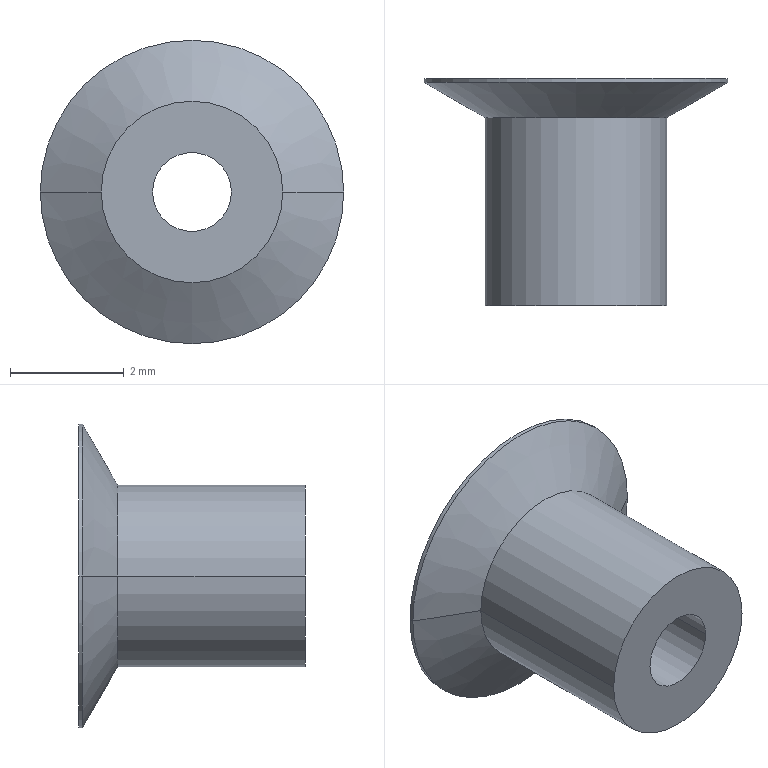Part | NX | features solid 2 | 1 solid | 12 faces | box 5.348 x 4 x 5.348 mm | volume 31.105 mm3 | cylinder 6 | torus 2 | plane 2 | cone 2 | commonest cylinder face diameters 1.39 x2 3.2 x2 5.348 x2
STEP:
#1=CARTESIAN_POINT('',(-257.575,146.75,-216.46));
#2=VERTEX_POINT('',#1);
#3=CARTESIAN_POINT('',(-258.965,146.75,-216.46));
#4=VERTEX_POINT('',#3);
#5=CARTESIAN_POINT('',(-258.27,146.75,-216.46));
#6=DIRECTION('',(0.,1.,0.));
#7=DIRECTION('',(1.,0.,0.));
#8=AXIS2_PLACEMENT_3D('',#5,#6,#7);
#9=CIRCLE('',#8,0.695);
#10=EDGE_CURVE('',#2,#4,#9,.T.);
#11=ORIENTED_EDGE('',*,*,#10,.T.);
#12=CARTESIAN_POINT('',(-258.965,143.06,-216.46));
#13=VERTEX_POINT('',#12);
#14=CARTESIAN_POINT('',(-258.965,146.75,-216.46));
#15=DIRECTION('',(0.,-1.,0.));
#16=VECTOR('',#15,1000.);
#17=LINE('',#14,#16);
#18=EDGE_CURVE('',#4,#13,#17,.T.);
#19=ORIENTED_EDGE('',*,*,#18,.T.);
#20=CARTESIAN_POINT('',(-257.575,143.06,-216.46));
#21=VERTEX_POINT('',#20);
#22=CARTESIAN_POINT('',(-258.27,143.06,-216.46));
#23=DIRECTION('',(0.,-1.,0.));
#24=DIRECTION('',(-1.,0.,0.));
#25=AXIS2_PLACEMENT_3D('',#22,#23,#24);
#26=CIRCLE('',#25,0.695);
#27=EDGE_CURVE('',#13,#21,#26,.T.);
#28=ORIENTED_EDGE('',*,*,#27,.T.);
#29=CARTESIAN_POINT('',(-257.575,146.75,-216.46));
#30=DIRECTION('',(0.,-1.,0.));
#31=VECTOR('',#30,1000.);
#32=LINE('',#29,#31);
#33=EDGE_CURVE('',#21,#2,#32,.F.);
#34=ORIENTED_EDGE('',*,*,#33,.T.);
#35=EDGE_LOOP('',(#11,#19,#28,#34));
#36=FACE_BOUND('',#35,.T.);
#37=CARTESIAN_POINT('',(-258.27,141.06,-216.46));
#38=DIRECTION('',(0.,-1.,0.));
#39=DIRECTION('',(1.,0.,0.));
#40=AXIS2_PLACEMENT_3D('',#37,#38,#39);
#41=CYLINDRICAL_SURFACE('',#40,0.695);
#42=ADVANCED_FACE('',(#36),#41,.F.);
#43=ORIENTED_EDGE('',*,*,#33,.F.);
#44=CARTESIAN_POINT('',(-258.27,143.06,-216.46));
#45=DIRECTION('',(0.,-1.,0.));
#46=DIRECTION('',(1.,0.,0.));
#47=AXIS2_PLACEMENT_3D('',#44,#45,#46);
#48=CIRCLE('',#47,0.695);
#49=EDGE_CURVE('',#21,#13,#48,.T.);
#50=ORIENTED_EDGE('',*,*,#49,.T.);
#51=ORIENTED_EDGE('',*,*,#18,.F.);
#52=CARTESIAN_POINT('',(-258.27,146.75,-216.46));
#53=DIRECTION('',(0.,1.,0.));
#54=DIRECTION('',(-1.,0.,0.));
#55=AXIS2_PLACEMENT_3D('',#52,#53,#54);
#56=CIRCLE('',#55,0.695);
#57=EDGE_CURVE('',#4,#2,#56,.T.);
#58=ORIENTED_EDGE('',*,*,#57,.T.);
#59=EDGE_LOOP('',(#43,#50,#51,#58));
#60=FACE_BOUND('',#59,.T.);
#61=CARTESIAN_POINT('',(-258.27,141.06,-216.46));
#62=DIRECTION('',(0.,-1.,0.));
#63=DIRECTION('',(1.,0.,0.));
#64=AXIS2_PLACEMENT_3D('',#61,#62,#63);
#65=CYLINDRICAL_SURFACE('',#64,0.695);
#66=ADVANCED_FACE('',(#60),#65,.F.);
#67=ORIENTED_EDGE('',*,*,#57,.F.);
#68=CARTESIAN_POINT('',(-259.275,147.06,-216.46));
#69=VERTEX_POINT('',#68);
#70=CARTESIAN_POINT('',(-259.275,146.75,-216.46));
#71=DIRECTION('',(0.,0.,1.));
#72=DIRECTION('',(1.,0.,0.));
#73=AXIS2_PLACEMENT_3D('',#70,#71,#72);
#74=CIRCLE('',#73,0.31);
#75=EDGE_CURVE('',#4,#69,#74,.T.);
#76=ORIENTED_EDGE('',*,*,#75,.T.);
#77=CARTESIAN_POINT('',(-257.265,147.06,-216.46));
#78=VERTEX_POINT('',#77);
#79=CARTESIAN_POINT('',(-258.27,147.06,-216.46));
#80=DIRECTION('',(0.,1.,0.));
#81=DIRECTION('',(-1.,0.,0.));
#82=AXIS2_PLACEMENT_3D('',#79,#80,#81);
#83=CIRCLE('',#82,1.005);
#84=EDGE_CURVE('',#69,#78,#83,.T.);
#85=ORIENTED_EDGE('',*,*,#84,.T.);
#86=CARTESIAN_POINT('',(-257.265,146.75,-216.46));
#87=DIRECTION('',(0.,0.,-1.));
#88=DIRECTION('',(-1.,0.,0.));
#89=AXIS2_PLACEMENT_3D('',#86,#87,#88);
#90=CIRCLE('',#89,0.31);
#91=EDGE_CURVE('',#78,#2,#90,.F.);
#92=ORIENTED_EDGE('',*,*,#91,.T.);
#93=EDGE_LOOP('',(#67,#76,#85,#92));
#94=FACE_BOUND('',#93,.T.);
#95=CARTESIAN_POINT('',(-258.27,146.75,-216.46));
#96=DIRECTION('',(0.,-1.,0.));
#97=DIRECTION('',(1.,0.,0.));
#98=AXIS2_PLACEMENT_3D('',#95,#96,#97);
#99=TOROIDAL_SURFACE('',#98,1.005,0.31);
#100=ADVANCED_FACE('',(#94),#99,.T.);
#101=ORIENTED_EDGE('',*,*,#91,.F.);
#102=CARTESIAN_POINT('',(-258.27,147.06,-216.46));
#103=DIRECTION('',(0.,1.,0.));
#104=DIRECTION('',(1.,0.,0.));
#105=AXIS2_PLACEMENT_3D('',#102,#103,#104);
#106=CIRCLE('',#105,1.005);
#107=EDGE_CURVE('',#78,#69,#106,.T.);
#108=ORIENTED_EDGE('',*,*,#107,.T.);
#109=ORIENTED_EDGE('',*,*,#75,.F.);
#110=ORIENTED_EDGE('',*,*,#10,.F.);
#111=EDGE_LOOP('',(#101,#108,#109,#110));
#112=FACE_BOUND('',#111,.T.);
#113=CARTESIAN_POINT('',(-258.27,146.75,-216.46));
#114=DIRECTION('',(0.,-1.,0.));
#115=DIRECTION('',(1.,0.,0.));
#116=AXIS2_PLACEMENT_3D('',#113,#114,#115);
#117=TOROIDAL_SURFACE('',#116,1.005,0.31);
#118=ADVANCED_FACE('',(#112),#117,.T.);
#119=CARTESIAN_POINT('',(-255.596,147.06,-216.46));
#120=VERTEX_POINT('',#119);
#121=CARTESIAN_POINT('',(-260.944,147.06,-216.46));
#122=VERTEX_POINT('',#121);
#123=CARTESIAN_POINT('',(-258.27,147.06,-216.46));
#124=DIRECTION('',(0.,-1.,0.));
#125=DIRECTION('',(1.,0.,0.));
#126=AXIS2_PLACEMENT_3D('',#123,#124,#125);
#127=CIRCLE('',#126,2.674);
#128=EDGE_CURVE('',#120,#122,#127,.T.);
#129=ORIENTED_EDGE('',*,*,#128,.F.);
#130=CARTESIAN_POINT('',(-258.27,147.06,-216.46));
#131=DIRECTION('',(0.,-1.,0.));
#132=DIRECTION('',(-1.,0.,0.));
#133=AXIS2_PLACEMENT_3D('',#130,#131,#132);
#134=CIRCLE('',#133,2.674);
#135=EDGE_CURVE('',#122,#120,#134,.T.);
#136=ORIENTED_EDGE('',*,*,#135,.F.);
#137=EDGE_LOOP('',(#129,#136));
#138=FACE_BOUND('',#137,.T.);
#139=ORIENTED_EDGE('',*,*,#84,.F.);
#140=ORIENTED_EDGE('',*,*,#107,.F.);
#141=EDGE_LOOP('',(#139,#140));
#142=FACE_BOUND('',#141,.T.);
#143=CARTESIAN_POINT('',(-255.596,147.06,-216.46));
#144=DIRECTION('',(0.,-1.,0.));
#145=DIRECTION('',(1.,0.,0.));
#146=AXIS2_PLACEMENT_3D('',#143,#144,#145);
#147=PLANE('',#146);
#148=ADVANCED_FACE('',(#138,#142),#147,.F.);
#149=CARTESIAN_POINT('',(-255.596,146.99,-216.46));
#150=VERTEX_POINT('',#149);
#151=CARTESIAN_POINT('',(-255.596,147.06,-216.46));
#152=DIRECTION('',(0.,-1.,0.));
#153=VECTOR('',#152,1000.);
#154=LINE('',#151,#153);
#155=EDGE_CURVE('',#120,#150,#154,.T.);
#156=ORIENTED_EDGE('',*,*,#155,.T.);
#157=CARTESIAN_POINT('',(-260.944,146.99,-216.46));
#158=VERTEX_POINT('',#157);
#159=CARTESIAN_POINT('',(-258.27,146.99,-216.46));
#160=DIRECTION('',(0.,1.,0.));
#161=DIRECTION('',(1.,0.,0.));
#162=AXIS2_PLACEMENT_3D('',#159,#160,#161);
#163=CIRCLE('',#162,2.674);
#164=EDGE_CURVE('',#150,#158,#163,.T.);
#165=ORIENTED_EDGE('',*,*,#164,.T.);
#166=CARTESIAN_POINT('',(-260.944,147.06,-216.46));
#167=DIRECTION('',(0.,-1.,0.));
#168=VECTOR('',#167,1000.);
#169=LINE('',#166,#168);
#170=EDGE_CURVE('',#158,#122,#169,.F.);
#171=ORIENTED_EDGE('',*,*,#170,.T.);
#172=ORIENTED_EDGE('',*,*,#135,.T.);
#173=EDGE_LOOP('',(#156,#165,#171,#172));
#174=FACE_BOUND('',#173,.T.);
#175=CARTESIAN_POINT('',(-258.27,141.06,-216.46));
#176=DIRECTION('',(0.,-1.,0.));
#177=DIRECTION('',(1.,0.,0.));
#178=AXIS2_PLACEMENT_3D('',#175,#176,#177);
#179=CYLINDRICAL_SURFACE('',#178,2.674);
#180=ADVANCED_FACE('',(#174),#179,.T.);
#181=ORIENTED_EDGE('',*,*,#128,.T.);
#182=ORIENTED_EDGE('',*,*,#170,.F.);
#183=CARTESIAN_POINT('',(-258.27,146.99,-216.46));
#184=DIRECTION('',(0.,1.,0.));
#185=DIRECTION('',(-1.,0.,0.));
#186=AXIS2_PLACEMENT_3D('',#183,#184,#185);
#187=CIRCLE('',#186,2.674);
#188=EDGE_CURVE('',#158,#150,#187,.T.);
#189=ORIENTED_EDGE('',*,*,#188,.T.);
#190=ORIENTED_EDGE('',*,*,#155,.F.);
#191=EDGE_LOOP('',(#181,#182,#189,#190));
#192=FACE_BOUND('',#191,.T.);
#193=CARTESIAN_POINT('',(-258.27,141.06,-216.46));
#194=DIRECTION('',(0.,-1.,0.));
#195=DIRECTION('',(1.,0.,0.));
#196=AXIS2_PLACEMENT_3D('',#193,#194,#195);
#197=CYLINDRICAL_SURFACE('',#196,2.674);
#198=ADVANCED_FACE('',(#192),#197,.T.);
#199=CARTESIAN_POINT('',(-256.67,146.37,-216.46));
#200=VERTEX_POINT('',#199);
#201=CARTESIAN_POINT('',(-259.87,146.37,-216.46));
#202=VERTEX_POINT('',#201);
#203=CARTESIAN_POINT('',(-258.27,146.37,-216.46));
#204=DIRECTION('',(0.,-1.,0.));
#205=DIRECTION('',(1.,0.,0.));
#206=AXIS2_PLACEMENT_3D('',#203,#204,#205);
#207=CIRCLE('',#206,1.6);
#208=EDGE_CURVE('',#200,#202,#207,.T.);
#209=ORIENTED_EDGE('',*,*,#208,.F.);
#210=CARTESIAN_POINT('',(-256.67,146.37,-216.46));
#211=DIRECTION('',(0.866,0.5,0.));
#212=VECTOR('',#211,1000.);
#213=LINE('',#210,#212);
#214=EDGE_CURVE('',#150,#200,#213,.F.);
#215=ORIENTED_EDGE('',*,*,#214,.F.);
#216=ORIENTED_EDGE('',*,*,#188,.F.);
#217=CARTESIAN_POINT('',(-259.87,146.37,-216.46));
#218=DIRECTION('',(-0.866,0.5,0.));
#219=VECTOR('',#218,1000.);
#220=LINE('',#217,#219);
#221=EDGE_CURVE('',#202,#158,#220,.T.);
#222=ORIENTED_EDGE('',*,*,#221,.F.);
#223=EDGE_LOOP('',(#209,#215,#216,#222));
#224=FACE_BOUND('',#223,.T.);
#225=CARTESIAN_POINT('',(-258.27,146.68,-216.46));
#226=DIRECTION('',(0.,1.,0.));
#227=DIRECTION('',(-1.,0.,0.));
#228=AXIS2_PLACEMENT_3D('',#225,#226,#227);
#229=CONICAL_SURFACE('',#228,2.137,1.047);
#230=ADVANCED_FACE('',(#224),#229,.T.);
#231=ORIENTED_EDGE('',*,*,#221,.T.);
#232=ORIENTED_EDGE('',*,*,#164,.F.);
#233=ORIENTED_EDGE('',*,*,#214,.T.);
#234=CARTESIAN_POINT('',(-258.27,146.37,-216.46));
#235=DIRECTION('',(0.,-1.,0.));
#236=DIRECTION('',(-1.,0.,0.));
#237=AXIS2_PLACEMENT_3D('',#234,#235,#236);
#238=CIRCLE('',#237,1.6);
#239=EDGE_CURVE('',#202,#200,#238,.T.);
#240=ORIENTED_EDGE('',*,*,#239,.F.);
#241=EDGE_LOOP('',(#231,#232,#233,#240));
#242=FACE_BOUND('',#241,.T.);
#243=CARTESIAN_POINT('',(-258.27,146.68,-216.46));
#244=DIRECTION('',(0.,1.,0.));
#245=DIRECTION('',(-1.,0.,0.));
#246=AXIS2_PLACEMENT_3D('',#243,#244,#245);
#247=CONICAL_SURFACE('',#246,2.137,1.047);
#248=ADVANCED_FACE('',(#242),#247,.T.);
#249=CARTESIAN_POINT('',(-256.67,143.06,-216.46));
#250=VERTEX_POINT('',#249);
#251=CARTESIAN_POINT('',(-256.67,146.37,-216.46));
#252=DIRECTION('',(0.,-1.,0.));
#253=VECTOR('',#252,1000.);
#254=LINE('',#251,#253);
#255=EDGE_CURVE('',#200,#250,#254,.T.);
#256=ORIENTED_EDGE('',*,*,#255,.T.);
#257=CARTESIAN_POINT('',(-259.87,143.06,-216.46));
#258=VERTEX_POINT('',#257);
#259=CARTESIAN_POINT('',(-258.27,143.06,-216.46));
#260=DIRECTION('',(0.,1.,0.));
#261=DIRECTION('',(1.,0.,0.));
#262=AXIS2_PLACEMENT_3D('',#259,#260,#261);
#263=CIRCLE('',#262,1.6);
#264=EDGE_CURVE('',#250,#258,#263,.T.);
#265=ORIENTED_EDGE('',*,*,#264,.T.);
#266=CARTESIAN_POINT('',(-259.87,146.37,-216.46));
#267=DIRECTION('',(0.,-1.,0.));
#268=VECTOR('',#267,1000.);
#269=LINE('',#266,#268);
#270=EDGE_CURVE('',#258,#202,#269,.F.);
#271=ORIENTED_EDGE('',*,*,#270,.T.);
#272=ORIENTED_EDGE('',*,*,#239,.T.);
#273=EDGE_LOOP('',(#256,#265,#271,#272));
#274=FACE_BOUND('',#273,.T.);
#275=CARTESIAN_POINT('',(-258.27,141.06,-216.46));
#276=DIRECTION('',(0.,-1.,0.));
#277=DIRECTION('',(1.,0.,0.));
#278=AXIS2_PLACEMENT_3D('',#275,#276,#277);
#279=CYLINDRICAL_SURFACE('',#278,1.6);
#280=ADVANCED_FACE('',(#274),#279,.T.);
#281=ORIENTED_EDGE('',*,*,#208,.T.);
#282=ORIENTED_EDGE('',*,*,#270,.F.);
#283=CARTESIAN_POINT('',(-258.27,143.06,-216.46));
#284=DIRECTION('',(0.,1.,0.));
#285=DIRECTION('',(-1.,0.,0.));
#286=AXIS2_PLACEMENT_3D('',#283,#284,#285);
#287=CIRCLE('',#286,1.6);
#288=EDGE_CURVE('',#258,#250,#287,.T.);
#289=ORIENTED_EDGE('',*,*,#288,.T.);
#290=ORIENTED_EDGE('',*,*,#255,.F.);
#291=EDGE_LOOP('',(#281,#282,#289,#290));
#292=FACE_BOUND('',#291,.T.);
#293=CARTESIAN_POINT('',(-258.27,141.06,-216.46));
#294=DIRECTION('',(0.,-1.,0.));
#295=DIRECTION('',(1.,0.,0.));
#296=AXIS2_PLACEMENT_3D('',#293,#294,#295);
#297=CYLINDRICAL_SURFACE('',#296,1.6);
#298=ADVANCED_FACE('',(#292),#297,.T.);
#299=ORIENTED_EDGE('',*,*,#288,.F.);
#300=ORIENTED_EDGE('',*,*,#264,.F.);
#301=EDGE_LOOP('',(#299,#300));
#302=FACE_BOUND('',#301,.T.);
#303=ORIENTED_EDGE('',*,*,#49,.F.);
#304=ORIENTED_EDGE('',*,*,#27,.F.);
#305=EDGE_LOOP('',(#303,#304));
#306=FACE_BOUND('',#305,.T.);
#307=CARTESIAN_POINT('',(-257.575,143.06,-216.46));
#308=DIRECTION('',(0.,1.,0.));
#309=DIRECTION('',(-1.,0.,0.));
#310=AXIS2_PLACEMENT_3D('',#307,#308,#309);
#311=PLANE('',#310);
#312=ADVANCED_FACE('',(#302,#306),#311,.F.);
#313=CLOSED_SHELL('',(#42,#66,#100,#118,#148,#180,#198,#230,#248,#280,#298,#312));
#314=MANIFOLD_SOLID_BREP('',#313);
#315=(LENGTH_UNIT()NAMED_UNIT(*)SI_UNIT(.MILLI.,.METRE.));
#316=UNCERTAINTY_MEASURE_WITH_UNIT(LENGTH_MEASURE(0.00001),#315,'','');
#317=(NAMED_UNIT(*)PLANE_ANGLE_UNIT()SI_UNIT($,.RADIAN.));
#318=(NAMED_UNIT(*)SI_UNIT($,.STERADIAN.)SOLID_ANGLE_UNIT());
#319=(GEOMETRIC_REPRESENTATION_CONTEXT(3)GLOBAL_UNCERTAINTY_ASSIGNED_CONTEXT((#316))GLOBAL_UNIT_ASSIGNED_CONTEXT((#315,#317,#318))REPRESENTATION_CONTEXT('',''));
#320=ADVANCED_BREP_SHAPE_REPRESENTATION('',(#314),#319);